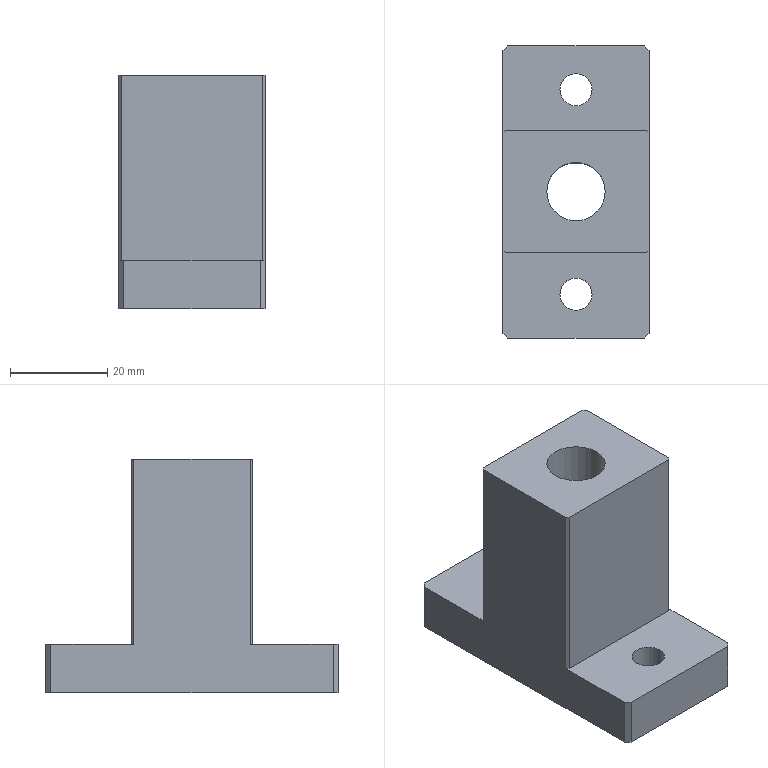NC program | NX | posted with a generic post | part box 30 x 60 x 48 mm
Lines 5020 to 6343 of 6343:
(PLANAR_MILL_1 , TOOL : D16精光)
N10032 T03 M6
N10034 G53
N10036 G17 G0 G90 X-16.313 Y-33.455 S2800 M3
N10038 G43 Z20. H3
N10040 Z-36.
N10042 G94 G1 Z-38. F600.
N10044 X-23.384 Y-26.384
N10046 X-23.884 Y-25.884
N10048 G2 X-28.6 Y-14.5 R16.1
N10050 G1 Y14.5
N10052 G2 X-23.884 Y25.884 R16.1
N10054 G1 X-23.384 Y26.384
N10056 X-16.313 Y33.455
N10058 Z-36.
N10060 G0 Z20.
N10062 X-11.275 Y-28.417
N10064 Z-36.
N10066 G1 Z-38.
N10068 X-17.728 Y-20.728
N10070 X-18.228 Y-20.228
N10072 G2 X-20.6 Y-14.5 R8.1
N10074 G1 Y14.5
N10076 G2 X-18.228 Y20.228 R8.1
N10078 G1 X-17.728 Y20.728
N10080 X-10.656 Y27.799
N10082 Z-36.
N10084 G0 Z20.
N10086 X16.313 Y33.455
N10088 Z-36.
N10090 G1 Z-38.
N10092 X23.384 Y26.384
N10094 X23.884 Y25.884
N10096 G2 X28.6 Y14.5 R16.1
N10098 G1 Y-14.5
N10100 G2 X23.884 Y-25.884 R16.1
N10102 G1 X23.384 Y-26.384
N10104 X16.313 Y-33.455
N10106 Z-36.
N10108 G0 Z20.
N10110 X10.656 Y27.799
N10112 Z-36.
N10114 G1 Z-38.
N10116 X17.728 Y20.728
N10118 X18.228 Y20.228
N10120 G2 X20.6 Y14.5 R8.1
N10122 G1 Y-14.5
N10124 G2 X18.228 Y-20.228 R8.1
N10126 G1 X17.728 Y-20.728
N10128 X10.656 Y-27.799
N10130 Z-36.
N10132 G0 Z20.
(PLANAR_MILL_1_COPY , TOOL : D16精光)
N10134 X-10.012 Y-28.547
N10136 Z-36.
N10138 G1 Z-38.
N10140 G41 X-10.586 Y-27.728 D3
N10142 X-17.657 Y-20.657
N10144 X-18.157 Y-20.157
N10146 G2 X-20.5 Y-14.5 R8.
N10148 G1 Y14.5
N10150 G2 X-18.157 Y20.157 R8.
N10152 G1 X-17.657 Y20.657
N10154 X-10.586 Y27.728
N10156 G40
N10158 X-10.012 Y28.547
N10160 Z-36.
N10162 G0 Z20.
N10164 Y-28.547
N10166 Z-36.
N10168 G1 Z-38.
N10170 G41 X-10.586 Y-27.728
N10172 X-17.657 Y-20.657
N10174 X-18.157 Y-20.157
N10176 G2 X-20.5 Y-14.5 R8.
N10178 G1 Y14.5
N10180 G2 X-18.157 Y20.157 R8.
N10182 G1 X-17.657 Y20.657
N10184 X-10.586 Y27.728
N10186 G40
N10188 X-10.012 Y28.547
N10190 Z-36.
N10192 G0 Z20.
N10194 X10.012
N10196 Z-36.
N10198 G1 Z-38.
N10200 G41 X10.586 Y27.728
N10202 X17.657 Y20.657
N10204 X18.157 Y20.157
N10206 G2 X20.5 Y14.5 R8.
N10208 G1 Y-14.5
N10210 G2 X18.157 Y-20.157 R8.
N10212 G1 X17.657 Y-20.657
N10214 X10.586 Y-27.728
N10216 G40
N10218 X10.012 Y-28.547
N10220 Z-36.
N10222 G0 Z20.
N10224 Y28.547
N10226 Z-36.
N10228 G1 Z-38.
N10230 G41 X10.586 Y27.728
N10232 X17.657 Y20.657
N10234 X18.157 Y20.157
N10236 G2 X20.5 Y14.5 R8.
N10238 G1 Y-14.5
N10240 G2 X18.157 Y-20.157 R8.
N10242 G1 X17.657 Y-20.657
N10244 X10.586 Y-27.728
N10246 G40
N10248 X10.012 Y-28.547
N10250 Z-36.
N10252 G0 Z20.
(PLANAR_MILL_2 , TOOL : D16精光)
N10254 X37.535 Y-23.174
N10256 Z-21.25
N10258 G1 Z-24.25
N10260 G41 X36.55 Y-23.
N10262 X28.999
N10264 X-29.
N10266 G2 X-34.657 Y-20.657 R8.
N10268 G1 X-35.657 Y-19.657
N10270 G2 X-38. Y-14. R8.
N10272 G1 Y14.
N10274 G2 X-35.657 Y19.657 R8.
N10276 G1 X-34.657 Y20.657
N10278 G2 X-29. Y23. R8.
N10280 G1 X29.
N10282 G2 X34.657 Y20.657 R8.
N10284 G1 X35.657 Y19.657
N10286 G2 X38. Y14. R8.
N10288 G1 Y-14.
N10290 G2 X35.657 Y-19.657 R8.
N10292 G1 X34.658 Y-20.656
N10294 X29.318 Y-25.995
N10296 G40
N10298 X28.745 Y-26.815
N10300 Z-21.25
N10302 G0 Z20.
N10304 X37.535 Y-23.174
N10306 Z-21.25
N10308 G1 Z-24.25
N10310 G41 X36.55 Y-23.
N10312 X28.999
N10314 X-29.
N10316 G2 X-34.657 Y-20.657 R8.
N10318 G1 X-35.657 Y-19.657
N10320 G2 X-38. Y-14. R8.
N10322 G1 Y14.
N10324 G2 X-35.657 Y19.657 R8.
N10326 G1 X-34.657 Y20.657
N10328 G2 X-29. Y23. R8.
N10330 G1 X29.
N10332 G2 X34.657 Y20.657 R8.
N10334 G1 X35.657 Y19.657
N10336 G2 X38. Y14. R8.
N10338 G1 Y-14.
N10340 G2 X35.657 Y-19.657 R8.
N10342 G1 X34.658 Y-20.656
N10344 X29.318 Y-25.995
N10346 G40
N10348 X28.745 Y-26.815
N10350 Z-21.25
N10352 G0 Z20.
N10354 X37.535 Y-23.174
N10356 Z-45.5
N10358 G1 Z-48.5
N10360 G41 X36.55 Y-23.
N10362 X28.999
N10364 X-29.
N10366 G2 X-34.657 Y-20.657 R8.
N10368 G1 X-35.657 Y-19.657
N10370 G2 X-38. Y-14. R8.
N10372 G1 Y14.
N10374 G2 X-35.657 Y19.657 R8.
N10376 G1 X-34.657 Y20.657
N10378 G2 X-29. Y23. R8.
N10380 G1 X29.
N10382 G2 X34.657 Y20.657 R8.
N10384 G1 X35.657 Y19.657
N10386 G2 X38. Y14. R8.
N10388 G1 Y-14.
N10390 G2 X35.657 Y-19.657 R8.
N10392 G1 X34.658 Y-20.656
N10394 X29.318 Y-25.995
N10396 G40
N10398 X28.745 Y-26.815
N10400 Z-45.5
N10402 G0 Z20.
N10404 X37.535 Y-23.174
N10406 Z-45.5
N10408 G1 Z-48.5
N10410 G41 X36.55 Y-23.
N10412 X28.999
N10414 X-29.
N10416 G2 X-34.657 Y-20.657 R8.
N10418 G1 X-35.657 Y-19.657
N10420 G2 X-38. Y-14. R8.
N10422 G1 Y14.
N10424 G2 X-35.657 Y19.657 R8.
N10426 G1 X-34.657 Y20.657
N10428 G2 X-29. Y23. R8.
N10430 G1 X29.
N10432 G2 X34.657 Y20.657 R8.
N10434 G1 X35.657 Y19.657
N10436 G2 X38. Y14. R8.
N10438 G1 Y-14.
N10440 G2 X35.657 Y-19.657 R8.
N10442 G1 X34.658 Y-20.656
N10444 X29.318 Y-25.995
N10446 G40
N10448 X28.745 Y-26.815
N10450 Z-45.5
N10452 G0 Z20.
N10454 M5
(DRILLING , TOOL : D6倒角刀)
N10456 T05 M6
N10458 G53
N10460 G17 G0 G90 X0. Y0. S1600 M3
N10462 G43 Z20. H5
N10464 G94 G81 G99 Z-2. F60. R3.
N10466 G80
N10468 G0 X0. Y0. Z20.
(DRILLING_COPY_1 , TOOL : D6倒角刀)
N10470 X-21.
N10472 G81 G98 Z-40. F60. R-35.
N10474 X21.
N10476 G80
N10478 G0 X21. Y0. Z20.
N10480 M5
(DRILLING_COPY , TOOL : D10.4钻头)
N10482 T10 M6
N10484 G53
N10486 G17 G0 G90 X0. Y0. S600 M3
N10488 G43 Z20. H10
N10490 G94 G83 G99 Z-52. F30. Q1.5 R3.
N10492 G80
N10494 G0 X0. Y0. Z20.
N10496 M5
(DRILLING_COPY_1_COPY , TOOL : D7钻头)
N10498 T12 M6
N10500 G53
N10502 G17 G0 G90 X-21. Y0. S1600 M3
N10504 G43 Z20. H12
N10506 G94 G81 G98 Z-52. F60. R-35.
N10508 X21.
N10510 G80
N10512 G0 X21. Y0. Z20.
N10514 M5
(PLANAR_MILL_3 , TOOL : D6倒角刀)
N10516 T05 M6
N10518 G53
N10520 G17 G0 G90 X2. Y-19. S3000 M3
N10522 G43 Z20. H5
N10524 Z0.
N10526 G94 G1 Z-2. F800.
N10528 G3 X0. Y-17. R2.
N10530 G1 X-12.
N10532 G2 X-13.414 Y-16.414 R2.
N10534 G1 X-13.914 Y-15.914
N10536 G2 X-14.5 Y-14.5 R2.
N10538 G1 Y14.5
N10540 G2 X-13.914 Y15.914 R2.
N10542 G1 X-13.414 Y16.414
N10544 G2 X-12. Y17. R2.
N10546 G1 X12.
N10548 G2 X13.414 Y16.414 R2.
N10550 G1 X13.914 Y15.914
N10552 G2 X14.5 Y14.5 R2.
N10554 G1 Y-14.5
N10556 G2 X13.914 Y-15.914 R2.
N10558 G1 X13.414 Y-16.414
N10560 G2 X12. Y-17. R2.
N10562 G1 X0.
N10564 G3 X-2. Y-19. R2.
N10566 G1 Z0.
N10568 G0 Z20.
(PLANAR_MILL_3_COPY_COPY , TOOL : D6倒角刀)
N10570 X-1. Y-3.04
N10572 Z0.
N10574 G1 Z-2.
N10576 Y-3.2
N10578 G3 X0. Y-4.2 R1.
N10580 X4.2 Y0. R4.2
N10582 X0. Y-4.2 R-4.2
N10584 X1. Y-3.2 R1.
N10586 G1 Y-3.04
N10588 Z0.
N10590 G0 Z20.
(PLANAR_MILL_3_COPY_COPY_1 , TOOL : D6倒角刀)
N10592 X-21. Y1.8
N10594 Z-39.5
N10596 G3 X-22.8 Y0. R1.8
N10598 X-21. Y1.8 R-1.8
N10600 G0 Z20.
N10602 X21.
N10604 Z-39.5
N10606 G3 X19.2 Y0. R1.8
N10608 X21. Y1.8 R-1.8
N10610 G0 Z20.
(PLANAR_MILL_3_COPY , TOOL : D6倒角刀)
N10612 X-15.2 Y-16.5
N10614 Z-39.5
N10616 G1 X-29.
N10618 G2 X-30.061 Y-16.061 R1.5
N10620 G1 X-31.061 Y-15.061
N10622 G2 X-31.5 Y-14. R1.5
N10624 G1 Y14.
N10626 G2 X-31.061 Y15.061 R1.5
N10628 G1 X-30.061 Y16.061
N10630 G2 X-29. Y16.5 R1.5
N10632 G1 X-15.2
N10634 G0 Z20.
N10636 X15.2
N10638 Z-39.5
N10640 G1 X29.
N10642 G2 X30.061 Y16.061 R1.5
N10644 G1 X31.061 Y15.061
N10646 G2 X31.5 Y14. R1.5
N10648 G1 Y-14.
N10650 G2 X31.061 Y-15.061 R1.5
N10652 G1 X30.061 Y-16.061
N10654 G2 X29. Y-16.5 R1.5
N10656 G1 X15.2
N10658 G0 Z20.
N10660 M5
(ADAPTIVE_MILLING_1 , TOOL : D16开粗)
N10662 T02 M6
N10664 G54
N10666 G17 G0 G90 X-33.882 Y-40.4 S3500 M3
N10668 G43 Z20. H2
N10670 Z3.1
N10672 G94 G1 X-33.733 Y-40.382 Z2.163 F2000.
N10674 X-33.584 Y-40.365 Z1.792
N10676 X-33.435 Y-40.348 Z1.52
N10678 X-33.286 Y-40.33 Z1.3
N10680 X-33.137 Y-40.313 Z1.116
N10682 X-32.988 Y-40.296 Z0.958
N10684 X-32.839 Y-40.278 Z0.82
N10686 X-32.69 Y-40.261 Z0.7
N10688 X-32.541 Y-40.244 Z0.595
N10690 X-32.392 Y-40.226 Z0.502
N10692 X-32.243 Y-40.209 Z0.421
N10694 X-32.094 Y-40.192 Z0.35
N10696 X-31.945 Y-40.174 Z0.29
N10698 X-31.796 Y-40.157 Z0.238
N10700 X-31.647 Y-40.14 Z0.195
N10702 X-31.498 Y-40.122 Z0.161
N10704 X-31.349 Y-40.105 Z0.134
N10706 X-31.2 Y-40.087 Z0.115
N10708 X-31.051 Y-40.07 Z0.104
N10710 X-30.902 Y-40.053 Z0.1
N10712 X-28.735 Y-39.801
N10714 G3 X-27.32 Y-37.984 R1.616
N10716 G2 X-27.629 Y-34.916 R14.337
N10718 X-27.7 Y-24.679 R454.28
N10720 G1 X-27.698 Y32.776
N10722 G2 X-24.199 Y39.696 R8.88
N10724 X-18.432 Y42.168 R13.003
N10726 X-12.196 Y42.66 R38.28
N10728 X-2.971 Y42.7 R675.708
N10730 G1 X17.776 Y42.698
N10732 G2 X24.766 Y39.11 R8.901
N10734 X27.195 Y33.284 R13.173
N10736 X27.657 Y27.308 R38.711
N10738 X27.7 Y18.083 R671.204
N10740 G1 X27.698 Y-32.758
N10742 G2 X24.24 Y-39.65 R8.875
N10744 X18.404 Y-42.169 R13.006
N10746 X12.543 Y-42.652 R36.738
N10748 X2.569 Y-42.7 R682.497
N10750 G1 X-17.639 Y-42.698
N10752 G2 X-24.141 Y-39.458 R8.854
N10754 X-26.803 Y-33.657 R12.752
N10756 X-27.343 Y-27.764 R34.072
N10758 X-27.399 Y-17.602 R654.893
N10760 G1 X-27.398 Y30.826
N10762 G2 X-22.489 Y39.631 R10.569
N10764 X-16.226 Y41.905 R15.742
N10766 X-9.385 Y42.362 R49.49
N10768 X0.253 Y42.399 R699.93
N10770 G1 X15.863 Y42.398
N10772 G2 X24.694 Y37.391 R10.583
N10774 X26.906 Y31.218 R15.839
N10776 X27.357 Y24.676 R48.015
N10778 X27.399 Y14.964 R688.44
N10780 G1 X27.398 Y-30.8
N10782 G2 X22.457 Y-39.645 R10.589
N10784 X16.292 Y-41.891 R15.715
N10786 X9.377 Y-42.362 R48.874
N10788 G1 X0.939 Y-42.399
N10790 X-15.5 Y-42.398
N10792 G2 X-24.321 Y-37.464 R10.611
N10794 X-26.587 Y-31.263 R15.768
N10796 X-27.058 Y-24.535 R47.839
N10798 X-27.099 Y-14.785 R694.891
N10800 G1 X-27.097 Y29.025
N10802 G2 X-20.817 Y39.661 R11.8
N10804 X-14.246 Y41.668 R18.49
N10806 X-6.837 Y42.07 R64.048
N10808 G1 X1.826 Y42.099
N10810 G2 X14.626 Y42.082 R953.08
N10812 X24.585 Y35.953 R11.744
N10814 X26.651 Y29.372 R18.24
N10816 X27.066 Y22.151 R60.772
N10818 G1 X27.099 Y13.338
N10820 X27.098 Y-29.001
N10822 G2 X20.771 Y-39.682 R11.82
N10824 X14.39 Y-41.646 R18.382
N10826 X6.832 Y-42.07 R62.487
N10828 G1 X-1.83 Y-42.099
N10830 G2 X-14.339 Y-42.08 R914.437
N10832 X-24.252 Y-35.977 R11.771
N10834 X-26.328 Y-29.474 R18.108
N10836 X-26.764 Y-22.142 R59.359
N10838 G1 X-26.798 Y-13.067
N10840 X-26.797 Y27.376
N10842 G2 X-25.614 Y33.4 R14.131
N10844 X-19.055 Y39.739 R12.995
N10846 X-12.359 Y41.434 R21.693
N10848 X-4.119 Y41.78 R85.393
N10850 G1 X2.893 Y41.798
N10852 G2 X13.275 Y41.777 R584.817
N10854 X24.362 Y34.824 R12.638
N10856 X26.34 Y28.131 R19.881
N10858 X26.769 Y20.198 R68.335
N10860 G1 X26.799 Y10.71
N10862 X26.797 Y-27.388
N10864 G2 X25.527 Y-33.578 R14.031
N10866 X18.963 Y-39.778 R13.057
N10868 X12.182 Y-41.451 R22.04
N10870 X4.054 Y-41.78 R88.174
N10872 G1 X-2.958 Y-41.798
N10874 G2 X-13.1 Y-41.769 R481.151
N10876 X-24.075 Y-34.771 R12.662
N10878 X-26.041 Y-28.076 R20.002
N10880 X-26.466 Y-20.292 R67.692
N10882 G1 X-26.498 Y-10.805
N10884 X-26.497 Y25.875
N10886 G2 X-25.724 Y31.421 R17.117
N10888 X-18.907 Y39.074 R13.338
N10890 X-11.899 Y41.047 R21.387
N10892 X-3.589 Y41.47 R75.571
N10894 X12.076 Y41.471 R773.369
N10896 X19.357 Y39.299 R13.939
N10898 X24.736 Y32.409 R14.185
N10900 X26.204 Y25.423 R25.464
N10902 X26.487 Y16.28 R118.068
N10904 G1 X26.498 Y8.855
N10906 X26.497 Y-25.851
N10908 G2 X25.741 Y-31.363 R17.219
N10910 X18.901 Y-39.073 R13.341
N10912 X12.044 Y-41.027 R21.236
N10914 X3.886 Y-41.466 R72.053
N10916 X-11.639 Y-41.475 R857.389
N10918 X-18.773 Y-39.466 R14.133
N10920 X-24.34 Y-32.623 R14.073
N10922 X-25.875 Y-25.69 R24.7
N10924 X-26.183 Y-16.96 R105.018
N10926 G1 X-26.198 Y-9.123
N10928 X-26.197 Y24.188
N10930 G2 X-25.715 Y29.478 R22.354
N10932 X-18.332 Y38.648 R13.811
N10934 X-11.299 Y40.687 R21.85
N10936 X-3.143 Y41.158 R70.407
N10938 X11.032 Y41.164 R516.672
N10940 X18.035 Y39.326 R15.164
N10942 X24.113 Y32.336 R14.378
N10944 X25.821 Y25.177 R24.491
N10946 X26.18 Y16.037 R99.272
N10948 G1 X26.198 Y7.375
N10950 X26.196 Y-24.5
N10952 G2 X25.589 Y-29.962 R20.319
N10954 X18.36 Y-38.631 R13.821
N10956 X11.371 Y-40.675 R21.753
N10958 X3.103 Y-41.158 R69.904
N10960 X-10.622 Y-41.167 R540.571
N10962 X-17.475 Y-39.457 R15.373
N10964 X-23.77 Y-32.408 R14.328
N10966 X-25.491 Y-25.404 R24.088
N10968 X-25.872 Y-16.866 R88.44
N10970 G1 X-25.897 Y-8.204
N10972 X-25.896 Y23.025
N10974 G2 X-25.449 Y28.433 R25.294
N10976 X-17.774 Y38.241 R14.284
N10978 X-10.46 Y40.367 R22.583
N10980 X-1.779 Y40.859 R74.378
N10982 X10.033 Y40.859 R373.006
N10984 X16.776 Y39.29 R16.437
N10986 X23.562 Y32.111 R14.626
N10988 X25.433 Y24.951 R23.97
N10990 X25.866 Y16.266 R82.968
N10992 G1 X25.898 Y5.954
N10994 X25.896 Y-23.076
N10996 G2 X25.421 Y-28.556 R24.726
N10998 X17.689 Y-38.281 R14.305
N11000 X10.481 Y-40.363 R22.655
N11002 X1.95 Y-40.857 R73.076
N11004 X-9.712 Y-40.858 R354.587
N11006 X-16.422 Y-39.306 R16.481
N11008 X-23.268 Y-32.073 R14.642
N11010 X-25.128 Y-24.951 R24.02
N11012 X-25.562 Y-16.454 R81.167
N11014 G1 X-25.597 Y-7.379
N11016 X-25.596 Y21.713
N11018 G2 X-25.196 Y27.352 R29.642
N11020 X-17.04 Y37.945 R14.759
N11022 X-9.788 Y40.034 R23.35
N11024 X-0.997 Y40.553 R74.139
N11026 X9.128 Y40.552 R269.659
N11028 X15.792 Y39.109 R17.564
N11030 X23.153 Y31.606 R14.98
N11032 X25.106 Y24.238 R24.504
N11034 X25.561 Y15.479 R82.657
N11036 X25.597 Y4.754 R754.156
N11038 G1 X25.596 Y-21.801
N11040 G2 X25.185 Y-27.401 R28.98
N11042 X17.019 Y-37.953 R14.766
N11044 X9.802 Y-40.03 R23.357
N11046 X1.01 Y-40.553 R73.772
N11048 X-8.964 Y-40.544 R232.213
N11050 X-15.783 Y-38.963 R17.237
N11052 X-22.859 Y-31.571 R15.034
N11054 X-24.778 Y-24.421 R24.333
N11056 X-25.255 Y-15.851 R77.983
N11058 X-25.297 Y-4.714 R754.607
N11060 G1 X-25.296 Y20.701
N11062 G2 X-24.903 Y26.492 R32.266
N11064 X-16.425 Y37.606 R15.179
N11066 X-8.993 Y39.724 R24.11
N11068 X-0.201 Y40.249 R75.555
N11070 X8.61 Y40.228 R166.339
N11072 X15.637 Y38.552 R17.755
N11074 X22.837 Y30.938 R15.432
N11076 X24.793 Y23.458 R25.361
N11078 X25.257 Y14.662 R84.012
N11080 X25.297 Y3.524 R761.56
N11082 G1 X25.296 Y-20.713
N11084 G2 X24.907 Y-26.467 R32.316
N11086 X16.472 Y-37.58 R15.176
N11088 X9.002 Y-39.721 R24.067
N11090 X0.286 Y-40.247 R74.816
N11092 X-8.301 Y-40.227 R157.879
N11094 X-15.328 Y-38.548 R17.773
N11096 X-22.552 Y-30.883 R15.459
N11098 X-24.483 Y-23.508 R25.359
N11100 X-24.959 Y-14.45 R84.449
N11102 X-24.996 Y-3.725 R751.569
N11104 G1 X-24.995 Y19.613
N11106 G2 X-24.635 Y25.52 R36.306
N11108 X-15.82 Y37.276 R15.579
N11110 X-8.42 Y39.389 R24.638
N11112 X0.595 Y39.945 R75.505
N11114 X8.28 Y39.89 R104.925
N11116 X15.647 Y37.907 R17.69
N11118 X22.575 Y30.174 R15.917
N11120 X24.499 Y22.567 R26.493
N11122 X24.964 Y13.058 R92.521
N11124 G1 X24.997 Y2.333
N11126 X24.995 Y-19.551
N11128 G2 X24.651 Y-25.422 R37.208
N11130 X15.76 Y-37.303 R15.598
N11132 X8.315 Y-39.402 R24.852
N11134 X-0.663 Y-39.946 R76.612
N11136 X-8.048 Y-39.883 R95.496
N11138 X-15.38 Y-37.88 R17.595
N11140 X-22.248 Y-30.216 R15.916
N11142 X-24.167 Y-22.796 R26.156
N11144 X-24.657 Y-13.477 R86.705
N11146 X-24.696 Y-2.339 R767.284
N11148 G1 X-24.695 Y18.451
N11150 G2 X-24.362 Y24.586 R41.171
N11152 X-18.998 Y34.514 R15.94
N11154 X-11.263 Y38.384 R19.174
N11156 X-3.289 Y39.486 R40.638
N11158 X7.169 Y39.6 R116.476
N11160 X14.291 Y37.968 R19.135
N11162 X22.066 Y29.987 R16.048
N11164 X24.118 Y22.415 R25.976
N11166 X24.651 Y13.023 R83.063
N11168 X24.696 Y1.473 R765.926
N11170 G1 X24.695 Y-18.463
N11172 G2 X24.359 Y-24.598 R40.906
N11174 X18.917 Y-34.58 R15.937
N11176 X11.241 Y-38.387 R19.231
N11178 X3.118 Y-39.495 R41.136
N11180 X-6.853 Y-39.598 R111.652
N11182 X-13.871 Y-38.016 R19.222
N11184 X-21.688 Y-30.133 R16.014
N11186 X-23.803 Y-22.497 R25.689
N11188 X-24.342 Y-13.519 R79.011
N11190 X-24.396 Y-1.556 R761.354
N11192 G1 X-24.395 Y17.288
N11194 G2 X-24.105 Y23.539 R47.819
N11196 X-20.426 Y32.234 R16.763
N11198 X-12.753 Y37.418 R17.605
N11200 X-4.835 Y39.016 R31.865
N11202 X6.705 Y39.269 R91.632
N11204 X13.987 Y37.516 R19.271
N11206 X21.669 Y29.57 R16.347
N11208 X23.79 Y21.858 R26.28
N11210 X24.342 Y12.655 R80.982
N11212 X24.396 Y0.28 R776.756
N11214 G1 X24.395 Y-17.301
N11216 G2 X24.102 Y-23.552 R47.524
N11218 X20.419 Y-32.239 R16.76
N11220 X12.586 Y-37.474 R17.673
N11222 X4.691 Y-39.028 R32.435
N11224 X-6.474 Y-39.261 R87.314
N11226 X-13.815 Y-37.446 R19.099
N11228 X-21.445 Y-29.386 R16.416
N11230 X-23.498 Y-21.771 R26.612
N11232 X-24.039 Y-12.717 R80.96
N11234 X-24.095 Y-0.342 R771.606
N11236 G1 X-24.094 Y16.576
N11238 G2 X-23.761 Y23.124 R47.129
N11240 X-19.887 Y31.978 R17.024
N11242 X-11.964 Y37.172 R18.087
N11244 X-4.109 Y38.712 R33.072
N11246 X6.193 Y38.938 R76.025
N11248 X13.574 Y37.122 R19.503
N11250 X21.368 Y28.964 R16.658
N11252 X23.503 Y21.027 R27.155
N11254 X24.047 Y11.41 R86.837
N11256 X24.096 Y-0.553 R775.233
N11258 G1 X24.094 Y-16.551
N11260 G2 X23.775 Y-23.025 R47.883
N11262 X20.048 Y-31.784 R17.111
N11264 X12.228 Y-37.076 R17.906
N11266 X4.124 Y-38.709 R32.574
N11268 X-6.065 Y-38.922 R71.54
N11270 X-13.661 Y-36.919 R19.083
N11272 X-21.092 Y-28.895 R16.727
N11274 X-23.184 Y-21.136 R27.098
N11276 X-23.737 Y-11.932 R82.4
N11278 X-23.795 Y0.855 R782.056
N11280 G1 X-23.794 Y15.451
N11282 G2 X-23.507 Y22.078 R54.417
N11284 X-20.391 Y30.423 R17.923
N11286 X-12.364 Y36.497 R17.669
N11288 X-4.261 Y38.325 R30.777
N11290 X5.999 Y38.58 R62.195
N11292 X13.812 Y36.396 R19.064
N11294 X21.123 Y28.251 R17.057
N11296 X23.214 Y20.222 R28.124
N11298 X23.74 Y10.979 R87.752
N11300 X23.795 Y-1.395 R775.593
N11302 G1 X23.794 Y-15.425
N11304 G2 X23.5 Y-22.127 R54.078
N11306 X20.272 Y-30.584 R17.849
N11308 X12.287 Y-36.524 R17.741
N11310 X4.295 Y-38.32 R30.86
N11312 X-5.777 Y-38.568 R59.496
N11314 X-13.617 Y-36.33 R18.919
N11316 X-20.845 Y-28.183 R17.099
N11318 X-22.901 Y-20.297 R28.152
N11320 X-23.443 Y-10.68 R88.672
N11322 X-23.495 Y1.695 R785.971
N11324 G1 X-23.494 Y14.363
N11326 G2 X-23.232 Y21.179 R61.509
N11328 X-20.498 Y29.288 R18.753
N11330 X-12.298 Y35.985 R17.638
N11332 X-4.233 Y37.949 R29.794
N11334 X5.686 Y38.224 R52.992
N11336 X13.772 Y35.799 R18.922
N11338 X20.801 Y27.72 R17.373
N11340 X22.893 Y19.69 R28.562
N11342 X23.439 Y10.148 R88.963
N11344 X23.495 Y-2.639 R791.621
N11346 G1 X23.494 Y-14.338
N11348 G2 X23.225 Y-21.229 R61.002
N11350 X20.472 Y-29.324 R18.713
N11352 X12.451 Y-35.917 R17.601
N11354 X4.438 Y-37.923 R29.304
N11356 X-5.293 Y-38.224 R51.68
N11358 X-13.395 Y-35.835 R18.993
N11360 X-20.488 Y-27.731 R17.359
N11362 X-22.583 Y-19.742 R28.491
N11364 X-23.143 Y-9.863 R90.015
N11366 X-23.194 Y2.512 R784.134
N11368 G1 X-23.193 Y13.726
N11370 G2 X-22.9 Y20.765 R60.237
N11372 X-20.049 Y28.99 R18.961
N11374 X-11.861 Y35.629 R17.902
N11376 X-3.766 Y37.623 R29.953
N11378 X5.552 Y37.844 R45.088
N11380 X13.952 Y35.051 R18.596
N11382 X20.549 Y27.041 R17.768
N11384 X22.59 Y19.032 R29.372
N11386 X23.141 Y9.227 R92.008
N11388 X23.195 Y-3.56 R795.695
N11390 X23.149 Y-17.225 R740.099
N11392 X22.27 Y-24.014 R28.594
N11394 X12.937 Y-35.138 R17.273
N11396 X4.863 Y-37.476 R27.255
N11398 X-5.234 Y-37.837 R44.383
N11400 X-13.755 Y-34.975 R18.536
N11402 X-20.279 Y-26.954 R17.816
N11404 X-22.298 Y-18.943 R29.617
N11406 X-22.843 Y-8.988 R94.149
N11408 X-22.894 Y3.387 R789.933
N11410 X-22.847 Y16.537 R684.946
N11412 X-21.966 Y23.44 R29.532
N11414 X-12.437 Y34.819 R17.523
N11416 X-4.138 Y37.187 R27.813
N11418 X5.323 Y37.465 R40.009
N11420 X14.299 Y34.152 R18.342
N11422 X20.44 Y26.021 R18.326
N11424 X22.367 Y17.717 R31.585
N11426 X22.853 Y7.532 R107.576
N11428 X22.894 Y-4.43 R799.748
N11430 X22.836 Y-16.85 R511.34
N11432 X21.849 Y-23.849 R28.004
N11434 X12.429 Y-34.82 R17.515
N11436 X4.24 Y-37.17 R27.692
N11438 X-5.145 Y-37.44 R38.539
N11440 X-14.221 Y-33.977 R18.184
N11442 X-20.203 Y-25.845 R18.448
N11444 X-22.06 Y-17.749 R31.83
N11446 X-22.551 Y-7.64 R106.146
N11448 X-22.594 Y4.322 R793.991
N11450 X-22.532 Y16.237 R460.867
N11452 X-21.528 Y23.347 R28.629
N11454 X-12.014 Y34.466 R17.734
N11456 X-3.609 Y36.868 R27.95
N11458 X5.55 Y37.02 R34.543
N11460 X15.434 Y32.506 R17.819
N11462 X20.525 Y24.423 R19.485
N11464 X22.158 Y16.164 R35.522
N11466 X22.566 Y5.488 R132.348
N11468 G1 X22.594 Y-4.412
N11470 G2 X22.536 Y-16.137 R477.907
N11472 X21.555 Y-23.251 R29.
N11474 X11.94 Y-34.499 R17.756
N11476 X3.562 Y-36.871 R28.04
N11478 X-5.41 Y-36.985 R33.173
N11480 X-15.839 Y-31.801 R17.645
N11482 X-20.474 Y-23.638 R20.201
N11484 X-21.932 Y-15.267 R38.828
N11486 X-22.273 Y-4.362 R157.775
N11488 G1 X-22.293 Y5.125
N11490 G2 X-22.218 Y15.9 R335.146
N11492 X-21.131 Y23.11 R28.208
N11494 X-11.598 Y34.113 R17.94
N11496 X-2.932 Y36.565 R28.059
N11498 X5.775 Y36.55 R30.197
N11500 X19.051 Y26.702 R17.682
N11502 X21.467 Y18.689 R27.575
N11504 X22.193 Y9.199 R74.063
N11506 X22.254 Y-14.788 R908.002
N11508 X21.455 Y-21.929 R33.425
N11510 X11.415 Y-34.198 R18.007
N11512 X2.473 Y-36.616 R28.53
N11514 X-6.042 Y-36.434 R28.22
N11516 X-18.618 Y-26.949 R17.597
N11518 X-21.144 Y-18.809 R27.177
N11520 X-21.89 Y-9.283 R72.732
N11522 X-21.942 Y14.513 R792.531
N11524 X-21.076 Y21.684 R32.542
N11526 X-11.099 Y33.805 R18.184
N11528 X-1.721 Y36.31 R28.255
N11530 X6.706 Y35.904 R25.724
N11532 X18.55 Y26.58 R17.692
N11534 X21.132 Y18.306 R27.358
N11536 X21.887 Y8.705 R73.318
N11538 X21.946 Y-14.356 R787.428
N11540 X21.114 Y-21.531 R33.333
N11542 X11.005 Y-33.848 R18.207
N11544 X1.317 Y-36.336 R28.308
N11546 X-7.2 Y-35.685 R24.087
N11548 X-18.206 Y-26.649 R17.651
N11550 X-20.797 Y-18.494 R27.078
N11552 X-21.581 Y-8.896 R71.172
N11554 X-21.644 Y13.753 R733.071
N11556 X-20.817 Y20.967 R34.207
N11558 X-10.615 Y33.494 R18.4
N11560 X4.645 Y35.83 R27.967
N11562 X18.221 Y26.125 R17.82
N11564 X20.81 Y17.849 R27.576
N11566 X21.576 Y8.4 R72.317
N11568 X21.641 Y-13.837 R677.085
N11570 X20.768 Y-21.157 R33.494
N11572 X10.536 Y-33.529 R18.405
N11574 X-4.397 Y-35.801 R27.393
N11576 X-17.843 Y-26.258 R17.767
N11578 X-20.468 Y-18.074 R27.208
N11580 X-21.27 Y-8.553 R70.157
N11582 X-21.34 Y13.195 R641.708
N11584 X-20.51 Y20.447 R34.864
N11586 X-10.04 Y33.229 R18.612
N11588 X4.419 Y35.405 R26.28
N11590 X17.749 Y25.947 R17.82
N11592 X20.43 Y17.74 R27.14
N11594 X21.268 Y7.997 R69.912
N11596 X21.333 Y-13.414 R573.947
N11598 X20.429 Y-20.768 R33.43
N11600 X10.15 Y-33.173 R18.576
N11602 X-4.223 Y-35.365 R25.707
N11604 X-17.428 Y-25.969 R17.771
N11606 X-20.135 Y-17.686 R27.158
N11608 X-20.962 Y-8.13 R69.427
N11610 X-21.036 Y12.644 R562.894
N11612 X-20.196 Y19.97 R35.401
N11614 X-9.586 Y32.907 R18.782
N11616 X4.216 Y34.967 R24.741
N11618 X17.315 Y25.696 R17.803
N11620 X20.095 Y17.371 R27.04
N11622 X20.947 Y7.967 R67.514
N11624 X21.024 Y-13.031 R482.993
N11626 X20.1 Y-20.345 R33.424
N11628 X9.512 Y-32.937 R18.777
N11630 X-3.964 Y-34.931 R24.252
N11632 X-16.897 Y-25.891 R17.723
N11634 X-19.745 Y-17.624 R26.568
N11636 X-20.642 Y-8.075 R65.675
N11638 X-20.726 Y12.323 R470.061
N11640 X-19.818 Y19.753 R34.67
N11642 X-9.103 Y32.599 R18.923
N11644 X4.111 Y34.503 R23.336
N11646 X16.799 Y25.588 R17.733
N11648 X19.732 Y17.16 R26.647
N11650 X20.637 Y7.611 R65.798
N11652 X20.725 Y-12.337 R444.846
N11654 X19.814 Y-19.766 R34.571
N11656 X9.022 Y-32.631 R18.924
N11658 X-3.836 Y-34.467 R22.888
N11660 X-16.453 Y-25.65 R17.667
N11662 X-19.365 Y-17.486 R26.235
N11664 X-20.316 Y-8.13 R62.216
N11666 X-20.416 Y11.967 R399.187
N11668 X-19.468 Y19.429 R34.359
N11670 X-8.39 Y32.391 R19.069
N11672 X3.972 Y34.032 R22.062
N11674 X16.3 Y25.443 R17.646
N11676 X19.326 Y17.161 R26.071
N11678 X20.311 Y7.658 R61.787
N11680 X20.416 Y-11.951 R381.208
N11682 X19.462 Y-19.45 R34.33
N11684 X8.31 Y-32.419 R19.056
N11686 X-3.91 Y-33.954 R21.574
N11688 X-15.978 Y-25.46 R17.58
N11690 X-19.001 Y-17.259 R25.929
N11692 X-20.005 Y-7.759 R60.929
N11694 X-20.103 Y11.663 R343.655
N11696 X-19.076 Y19.265 R33.613
N11698 X-7.613 Y32.198 R19.168
N11700 X4.298 Y33.462 R20.761
N11702 X15.812 Y25.268 R17.545
N11704 X18.943 Y17.03 R25.656
N11706 X19.972 Y7.909 R58.147
N11708 X20.1 Y-11.737 R319.243
N11710 X19.055 Y-19.336 R33.264
N11712 X7.405 Y-32.272 R19.149
N11714 X-4.263 Y-33.367 R20.29
N11716 X-15.527 Y-25.222 R17.488
N11718 X-18.686 Y-16.795 R25.867
N11720 X-19.69 Y-7.483 R60.35
N11722 X-19.796 Y11.226 R304.863
N11724 X-18.749 Y18.863 R33.751
N11726 X-6.305 Y32.18 R19.261
N11728 X5.242 Y32.7 R19.364
N11730 X15.565 Y24.696 R17.547
N11732 X18.671 Y16.36 R26.056
N11734 X19.691 Y6.899 R60.863
N11736 X19.794 Y-11.247 R291.019
N11738 X18.762 Y-18.811 R33.795
N11740 X5.902 Y-32.298 R19.23
N11742 X-5.718 Y-32.427 R18.808
N11744 X-15.366 Y-24.506 R17.574
N11746 X-18.386 Y-16.259 R26.277
N11748 X-19.395 Y-6.76 R61.621
N11750 X-19.496 Y10.599 R282.611
N11752 X-18.454 Y18.35 R34.57
N11754 X-3.681 Y32.416 R19.305
N11756 X8.707 Y30.683 R17.621
N11758 X15.99 Y22.905 R18.309
N11760 X18.607 Y14.558 R28.847
N11762 X19.452 Y4.627 R74.401
N11764 X19.491 Y-10.709 R268.259
N11766 X18.414 Y-18.491 R34.015
N11768 X-2.609 Y-32.601 R19.176
N11770 X-14.418 Y-25.044 R17.107
N11772 X-17.826 Y-16.916 R24.513
N11774 X-19.03 Y-7.516 R53.636
N11776 X-19.175 Y10.478 R237.708
N11778 X-18.065 Y18.181 R33.532
N11780 X-0.385 Y32.318 R19.116
N11782 X14.042 Y25.126 R16.916
N11784 X17.743 Y16.768 R23.972
N11786 X19.004 Y7.416 R51.806
N11788 X19.178 Y-10.391 R228.176
N11790 X18.046 Y-18.241 R33.59
N11792 X6.621 Y-30.985 R19.071
N11794 X-5.954 Y-31.172 R17.478
N11796 X-14.649 Y-23.724 R17.444
N11798 X-17.731 Y-15.468 R26.152
N11800 X-18.768 Y-6.16 R60.063
N11802 X-18.862 Y10.148 R214.335
N11804 X-17.712 Y17.882 R33.277
N11806 X-8.865 Y29.366 R19.151
N11808 X4.023 Y31.328 R17.633
N11810 X14.075 Y24.163 R16.989
N11812 X17.516 Y15.947 R24.671
N11814 X18.719 Y6.586 R54.059
N11816 X18.862 Y-10.134 R203.608
N11818 X17.704 Y-17.904 R33.217
N11820 X9.573 Y-28.925 R19.125
N11822 X-3.387 Y-31.345 R17.479
N11824 X-13.635 Y-24.336 R16.825
N11826 X-17.156 Y-16.166 R24.255
N11828 X-18.395 Y-6.96 R52.133
N11830 X-18.548 Y9.833 R189.027
N11832 X-17.345 Y17.635 R32.902
N11834 X-9.539 Y28.347 R19.135
N11836 X3.594 Y30.845 R17.114
N11838 X13.625 Y23.893 R16.77
N11840 X17.162 Y15.654 R24.362
N11842 X18.394 Y6.448 R52.647
N11844 X18.535 Y-10.046 R177.463
N11846 X17.237 Y-17.981 R31.831
N11848 X9.025 Y-28.652 R18.935
N11850 X-4.195 Y-30.549 R16.719
N11852 X-13.448 Y-23.678 R16.798
N11854 X-16.925 Y-15.359 R24.674
N11856 X-18.117 Y-5.996 R54.665
N11858 X-18.228 Y9.598 R169.291
N11860 X-16.932 Y17.534 R32.142
N11862 X-9.486 Y27.755 R19.011
N11864 X3.691 Y30.223 R16.512
N11866 X13.235 Y23.526 R16.599
N11868 X16.794 Y15.418 R24.049
N11870 X18.068 Y6.294 R51.084
N11872 X18.222 Y-9.673 R160.543
N11874 X16.884 Y-17.678 R31.704
N11876 X9.571 Y-27.677 R18.892
N11878 X-3.647 Y-30.087 R16.266
N11880 X-12.988 Y-23.412 R16.534
N11882 X-16.526 Y-15.256 R24.153
N11884 X-17.795 Y-5.829 R52.683
N11886 X-17.91 Y9.314 R152.107
N11888 X-16.553 Y17.315 R31.702
N11890 X-9.61 Y27.027 R18.904
N11892 X3.515 Y29.651 R16.003
N11894 X12.826 Y23.179 R16.379
N11896 X16.445 Y15.095 R23.762
N11898 X17.748 Y6.051 R50.069
N11900 X17.897 Y-9.503 R143.205
N11902 X16.468 Y-17.566 R30.919
N11904 X9.514 Y-27.07 R18.701
N11906 X-3.969 Y-29.368 R15.72
N11908 X-12.75 Y-22.819 R16.438
N11910 X-16.234 Y-14.706 R24.22
N11912 X-17.48 Y-5.502 R52.439
N11914 X-17.598 Y8.928 R138.646
N11916 X-16.218 Y16.963 R31.647
N11918 X-9.87 Y26.171 R18.83
N11920 X3.241 Y29.087 R15.556
N11922 X12.419 Y22.818 R16.134
N11924 X16.086 Y14.808 R23.41
N11926 X17.432 Y5.733 R49.071
N11928 X17.586 Y-9.071 R131.359
N11930 X16.171 Y-17.098 R31.124
N11932 X9.888 Y-26.131 R18.664
N11934 X-3.272 Y-28.918 R15.322
N11936 X-12.173 Y-22.696 R16.075
N11938 X-15.823 Y-14.629 R23.493
N11940 X-17.137 Y-5.624 R49.614
N11942 X-17.265 Y8.842 R123.495
N11944 X-15.811 Y16.825 R30.748
N11946 X-9.754 Y25.579 R18.564
N11948 X3.85 Y28.271 R15.054
N11950 X12.4 Y21.91 R16.144
N11952 X15.922 Y13.755 R24.071
N11954 X17.177 Y4.476 R52.776
N11956 X17.261 Y-8.867 R118.141
N11958 X15.727 Y-17.06 R30.291
N11960 X9.569 Y-25.688 R18.289
N11962 X-9.653 Y-24.676 R14.799
N11964 X-14.581 Y-17.104 R19.716
N11966 X-16.516 Y-8.606 R35.777
N11968 X-16.937 Y8.658 R108.92
N11970 X-15.333 Y16.875 R29.784
N11972 X-9.273 Y25.253 R18.083
N11974 X9.408 Y24.422 R14.597
N11976 X14.472 Y16.911 R19.384
N11978 X16.487 Y8.353 R34.987
N11980 X16.921 Y-8.834 R103.899
N11982 X15.32 Y-16.901 R29.374
N11984 X9.397 Y-25.12 R17.929
N11986 X-9.032 Y-24.42 R14.435
N11988 X-14.117 Y-17.001 R19.156
N11990 X-16.15 Y-8.604 R34.222
N11992 X-16.602 Y8.542 R98.84
N11994 X-14.954 Y16.636 R29.112
N11996 X-9.171 Y24.626 R17.729
N11998 X8.666 Y24.245 R14.228
N12000 X13.94 Y16.956 R18.684
N12002 X16.078 Y8.662 R32.766
N12004 X16.766 Y-4.135 R93.964
N12006 X16.113 Y-12.386 R47.947
N12008 X12.886 Y-20.652 R21.57
N12010 X4.44 Y-26.934 R15.316
N12012 X-8.625 Y-23.951 R14.145
N12014 X-13.727 Y-16.693 R18.784
N12016 X-15.819 Y-8.308 R33.429
N12018 X-16.276 Y8.275 R91.021
N12020 X-14.573 Y16.395 R28.605
N12022 X-8.965 Y24.06 R17.282
N12024 X8.08 Y23.9 R13.88
N12026 X13.537 Y16.661 R18.214
N12028 X15.748 Y8.341 R31.971
N12030 X16.252 Y-8.499 R86.457
N12032 X14.471 Y-16.64 R27.842
N12034 X8.902 Y-24.052 R16.937
N12036 X-7.672 Y-23.893 R13.719
N12038 X-13.143 Y-16.813 R17.931
N12040 X-15.415 Y-8.518 R31.214
N12042 X-15.925 Y8.282 R82.338
N12044 X-14.143 Y16.268 R27.562
N12046 X-8.646 Y23.561 R16.7
N12048 X7.521 Y23.502 R13.542
N12050 X13.049 Y16.535 R17.664
N12052 X15.358 Y8.408 R30.39
N12054 X15.896 Y-8.537 R78.343
N12056 X14.008 Y-16.576 R26.702
N12058 X8.414 Y-23.659 R16.251
N12060 X-7.191 Y-23.424 R13.393
N12062 X-12.747 Y-16.473 R17.501
N12064 X-15.077 Y-8.234 R30.363
N12066 X-15.575 Y8.226 R75.369
N12068 X-13.701 Y16.15 R26.553
N12070 X-8.139 Y23.17 R15.996
N12072 X7.065 Y22.999 R13.227
N12074 X12.625 Y16.241 R17.219
N12076 X15.021 Y8.1 R29.471
N12078 X15.581 Y-8.094 R73.093
N12080 X13.729 Y-16.062 R26.58
N12082 X8.338 Y-22.953 R15.819
N12084 X-6.638 Y-22.975 R13.077
N12086 X-12.263 Y-16.295 R16.961
N12088 X-14.714 Y-8.092 R29.082
N12090 X-15.239 Y7.988 R69.583
N12092 X-13.292 Y15.934 R25.776
N12094 X-7.762 Y22.655 R15.334
N12096 X6.664 Y22.432 R12.929
N12098 X12.308 Y15.705 R16.879
N12100 X14.7 Y7.682 R28.946
N12102 X15.217 Y-8.135 R66.831
N12104 X13.251 Y-15.996 R25.252
N12106 X7.649 Y-22.633 R14.997
N12108 X-6.255 Y-22.381 R12.787
N12110 X-11.928 Y-15.785 R16.612
N12112 X-14.355 Y-7.891 R28.207
N12114 X-14.895 Y7.809 R64.144
N12116 X-12.93 Y15.594 R24.949
N12118 X-7.366 Y22.119 R14.697
N12120 X6.232 Y21.858 R12.643
N12122 X11.948 Y15.24 R16.475
N12124 X14.376 Y7.268 R28.236
N12126 X14.864 Y-8.022 R61.531
N12128 X12.919 Y-15.58 R24.382
N12130 X7.372 Y-22.007 R14.407
N12132 X-5.934 Y-21.719 R12.512
N12134 X-11.645 Y-15.154 R16.309
N12136 X-14.092 Y-7.1 R28.117
N12138 X-14.532 Y7.779 R59.023
N12140 X-12.591 Y15.184 R23.89
N12142 X-6.985 Y21.537 R14.075
N12144 X5.955 Y21.155 R12.381
N12146 X11.634 Y14.663 R16.158
N12148 X14.064 Y6.766 R27.671
N12150 X14.501 Y-7.96 R56.535
N12152 X12.539 Y-15.248 R23.201
N12154 X6.783 Y-21.523 R13.709
N12156 X-5.749 Y-20.945 R12.272
N12158 X-11.323 Y-14.582 R16.019
N12160 X-13.757 Y-6.725 R27.33
N12162 X-14.159 Y7.776 R54.069
N12164 X-12.133 Y14.999 R22.408
N12166 X-6.124 Y21.164 R13.278
N12168 X5.922 Y20.269 R12.179
N12170 X11.433 Y13.84 R16.024
N12172 X13.781 Y6.077 R27.535
N12174 X14.159 Y-7.678 R52.365
N12176 X12.201 Y-14.804 R22.223
N12178 X6.3 Y-20.926 R13.094
N12180 X-5.583 Y-20.131 R12.05
N12182 X-11.147 Y-13.699 R15.845
N12184 X-13.512 Y-5.788 R27.496
N12186 X-13.821 Y7.445 R50.127
N12188 X-11.856 Y14.415 R21.546
N12190 X-5.772 Y20.468 R12.762
N12192 X5.722 Y19.463 R11.952
N12194 X11.197 Y13.064 R15.779
N12196 X13.542 Y5.07 R27.562
N12198 X13.773 Y-7.714 R47.743
N12200 X11.715 Y-14.615 R20.46
N12202 X4.925 Y-20.627 R12.312
N12204 X-5.798 Y-19.035 R11.937
N12206 X-11.079 Y-12.558 R15.929
N12208 X-13.294 Y-4.6 R28.146
N12210 X-13.431 Y7.477 R45.535
N12212 X-11.38 Y14.185 R19.749
N12214 X-4.247 Y20.145 R12.024
N12216 X6.08 Y18.245 R11.89
N12218 X11.208 Y11.736 R16.004
N12220 X13.325 Y3.83 R28.454
N12222 X13.396 Y-7.612 R43.389
N12224 X11.342 Y-14.16 R18.987
N12226 X3.603 Y-20.094 R11.735
N12228 X-6.272 Y-17.688 R11.918
N12230 X-11.095 Y-11.175 R16.24
N12232 X-13.091 Y-3.158 R29.245
N12234 X-13.007 Y7.647 R40.578
N12236 X-10.834 Y14.001 R17.659
N12238 X-1.406 Y19.671 R11.367
N12240 X7.43 Y16.08 R12.246
N12242 X11.589 Y9.361 R17.371
N12244 X13.278 Y0.473 R33.089
N12246 X12.844 Y-8.455 R35.467
N12248 X10.318 Y-14.662 R15.737
N12250 X-4.054 Y-18.092 R11.166
N12252 X-9.918 Y-12.246 R14.339
N12254 X-12.464 Y-4.669 R23.745
N12256 X-12.662 Y7.242 R37.686
N12258 X-10.5 Y13.393 R16.446
N12260 X4.046 Y17.454 R11.045
N12262 X9.965 Y11.58 R14.189
N12264 X12.481 Y3.997 R23.544
N12266 X12.607 Y-7.428 R35.631
N12268 X10.252 Y-13.622 R15.377
N12270 X-3.692 Y-17.234 R10.906
N12272 X-9.643 Y-11.438 R13.973
N12274 X-12.16 Y-3.935 R22.981
N12276 X-12.267 Y7.078 R33.788
N12278 X-9.931 Y13.075 R14.732
N12280 X3.547 Y16.634 R10.762
N12282 X9.567 Y10.965 R13.704
N12284 X12.127 Y3.522 R22.26
N12286 X12.254 Y-6.968 R32.163
N12288 X9.855 Y-12.994 R14.128
N12290 X-3.265 Y-16.351 R10.636
N12292 X-9.271 Y-10.752 R13.524
N12294 X-11.814 Y-3.371 R21.793
N12296 X-11.903 Y6.633 R30.238
N12298 X-9.329 Y12.676 R13.319
N12300 X3.142 Y15.708 R10.495
N12302 X9.217 Y10.214 R13.272
N12304 X11.827 Y2.632 R21.324
N12306 X11.834 Y-6.774 R28.002
N12308 X9.013 Y-12.817 R12.473
N12310 X-2.944 Y-15.358 R10.38
N12312 X-8.948 Y-9.926 R13.124
N12314 X-11.505 Y-2.478 R20.823
N12316 X-11.51 Y6.22 R26.256
N12318 X-8.614 Y12.258 R11.98
N12320 X2.911 Y14.642 R10.25
N12322 X8.975 Y9.22 R12.94
N12324 X11.529 Y1.581 R20.487
N12326 X11.421 Y-6.368 R23.735
N12328 X7.92 Y-12.64 R11.168
N12330 X-2.982 Y-14.141 R10.179
N12332 X-8.876 Y-8.604 R12.937
N12334 X-11.287 Y-0.648 R20.587
N12336 X-10.997 Y6.177 R20.62
N12338 X-6.454 Y12.766 R10.458
N12340 X3.714 Y13.023 R10.186
N12342 X9.278 Y7.156 R13.176
N12344 X11.356 Y-1.908 R21.137
N12346 X10.423 Y-7.644 R14.693
N12348 X-2.004 Y-13.245 R9.785
N12350 X-8.354 Y-7.958 R12.23
N12352 X-10.883 Y0.137 R18.717
N12354 X-10.391 Y6.08 R15.501
N12356 X1.908 Y12.444 R9.621
N12358 X8.31 Y7.273 R11.961
N12360 X10.695 Y-4.188 R17.734
N12362 X5.541 Y-11.452 R9.589
N12364 X-4.001 Y-10.899 R9.905
N12366 X-9.126 Y-4.707 R12.933
N12368 X-10.321 Y3.219 R16.113
N12370 X-3.498 Y11.163 R9.217
N12372 X5.216 Y9.175 R10.059
N12374 X9.656 Y2.308 R13.386
N12376 X10.03 Y-3.697 R12.686
N12378 X-0.309 Y-10.687 R8.916
N12380 X-7.365 Y-6.031 R10.845
N12382 X-9.668 Y1.299 R12.652
N12384 X-0.335 Y9.625 R8.561
N12386 X7.107 Y5.344 R10.301
N12388 X9.23 Y-0.379 R10.409
N12390 X1.959 Y-8.58 R8.003
N12392 X-7.17 Y-3.66 R9.3
N12394 X-6.591 Y3.172 R6.704
N12396 X-2.8 Y6.25 R8.687
N12398 G1 X-2.663 Y6.311 Z0.104
N12400 X-2.526 Y6.372 Z0.115
N12402 X-2.389 Y6.433 Z0.134
N12404 X-2.252 Y6.494 Z0.161
N12406 X-2.115 Y6.555 Z0.195
N12408 X-1.978 Y6.616 Z0.238
N12410 X-1.841 Y6.677 Z0.29
N12412 X-1.704 Y6.738 Z0.35
N12414 X-1.567 Y6.798 Z0.421
N12416 X-1.43 Y6.859 Z0.502
N12418 X-1.293 Y6.92 Z0.595
N12420 X-1.156 Y6.981 Z0.7
N12422 X-1.018 Y7.042 Z0.82
N12424 X-0.881 Y7.103 Z0.958
N12426 X-0.744 Y7.164 Z1.116
N12428 X-0.607 Y7.225 Z1.3
N12430 X-0.47 Y7.286 Z1.52
N12432 X-0.333 Y7.347 Z1.792
N12434 X-0.196 Y7.408 Z2.163
N12436 X-0.059 Y7.469 Z3.1
N12438 G0 Z20.
N12440 M5
(PLANAR_MILL_4 , TOOL : D50面刀)
N12442 T01 M6
N12444 G54
N12446 G17 G0 G90 X0. Y-57. S1600 M3
N12448 G43 Z20. H1
N12450 Z3.
N12452 G94 G1 Z0. F600.
N12454 Y-29.
N12456 Y29.
N12458 Y57.
N12460 Z3.
N12462 G0 Z20.
N12464 M5
(PLANAR_MILL_5 , TOOL : D6倒角刀)
N12466 T05 M6
N12468 G54
N12470 G17 G0 G90 X-20. Y0. S3000 M3
N12472 G43 Z20. H5
N12474 Z1.
N12476 G94 G1 Z-2. F1000.
N12478 X-17.
N12480 Y29.
N12482 G2 X-16.414 Y30.414 R2.
N12484 G1 X-15.414 Y31.414
N12486 G2 X-14. Y32. R2.
N12488 G1 X14.
N12490 G2 X15.414 Y31.414 R2.
N12492 G1 X16.414 Y30.414
N12494 G2 X17. Y29. R2.
N12496 G1 Y-29.
N12498 G2 X16.414 Y-30.414 R2.
N12500 G1 X15.414 Y-31.414
N12502 G2 X14. Y-32. R2.
N12504 G1 X-14.
N12506 G2 X-15.414 Y-31.414 R2.
N12508 G1 X-16.414 Y-30.414
N12510 G2 X-17. Y-29. R2.
N12512 G1 Y0.
N12514 X-20.
N12516 Z1.
N12518 G0 Z20.
(PLANAR_MILL_5_COPY , TOOL : D6倒角刀)
N12520 X-0.086 Y21.287
N12522 Z0.
N12524 G1 Z-2.
N12526 X-0.3 Y22.
N12528 G3 X-1.3 Y21. R1.
N12530 X0. Y19.7 R1.3
N12532 X-1.3 Y21. R-1.3
N12534 X-0.3 Y20. R1.
N12536 G1 X-0.086 Y20.713
N12538 Z0.
N12540 G0 Z20.
N12542 X-2.828 Y1.
N12544 Z0.
N12546 G1 Z-2.
N12548 X-3.
N12550 G3 X-4. Y0. R1.
N12552 X0. Y-4. R4.
N12554 X-4. Y0. R-4.
N12556 X-3. Y-1. R1.
N12558 G1 X-2.828
N12560 Z0.
N12562 G0 Z20.
N12564 X-0.086 Y-20.713
N12566 Z0.
N12568 G1 Z-2.
N12570 X-0.3 Y-20.
N12572 G3 X-1.3 Y-21. R1.
N12574 X0. Y-22.3 R1.3
N12576 X-1.3 Y-21. R-1.3
N12578 X-0.3 Y-22. R1.
N12580 G1 X-0.086 Y-21.287
N12582 Z0.
N12584 G0 Z20.
N12586 M5
N12588 M2